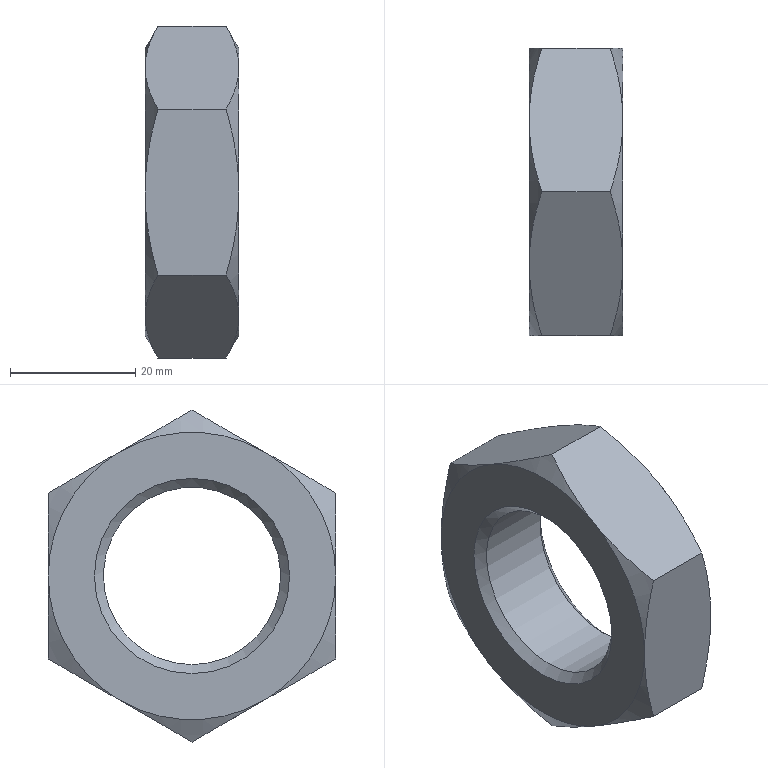Part | STEP file | Tube feed_id694_x_t | 1 solid | 23 faces | box 15 x 46 x 53.116 mm | volume 17601 mm3 | cone 14 | plane 8 | cylinder 1 | commonest cylinder face diameters 28.376 x1